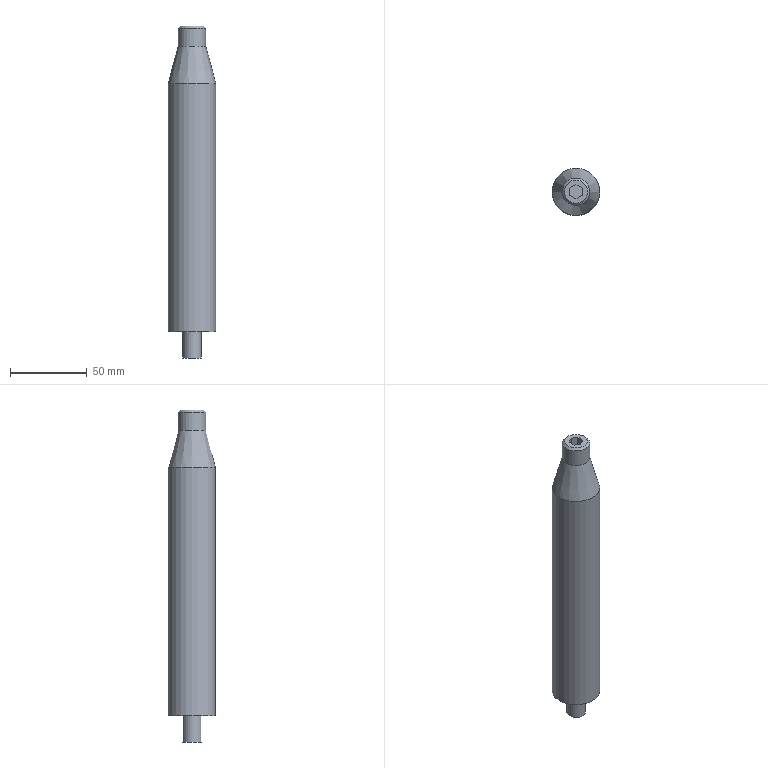Part | NX | features solid 2 | 1 solid | 15 faces | box 31 x 31 x 217 mm | volume 139271 mm3 | plane 10 | cylinder 3 | cone 2 | commonest cylinder face diameters 12 x1 18 x1 31 x1
STEP:
#1=CARTESIAN_POINT('',(-6.,-390.,130.));
#2=VERTEX_POINT('',#1);
#3=CARTESIAN_POINT('',(0.,-390.,130.));
#4=DIRECTION('',(0.,0.,-1.));
#5=DIRECTION('',(-1.,0.,0.));
#6=AXIS2_PLACEMENT_3D('',#3,#4,#5);
#7=CIRCLE('',#6,6.);
#8=EDGE_CURVE('',#2,#2,#7,.T.);
#9=ORIENTED_EDGE('',*,*,#8,.T.);
#10=EDGE_LOOP('',(#9));
#11=FACE_BOUND('',#10,.T.);
#12=CARTESIAN_POINT('',(-6.,-390.,113.));
#13=VERTEX_POINT('',#12);
#14=CARTESIAN_POINT('',(0.,-390.,113.));
#15=DIRECTION('',(0.,0.,-1.));
#16=DIRECTION('',(-1.,0.,0.));
#17=AXIS2_PLACEMENT_3D('',#14,#15,#16);
#18=CIRCLE('',#17,6.);
#19=EDGE_CURVE('',#13,#13,#18,.F.);
#20=ORIENTED_EDGE('',*,*,#19,.T.);
#21=EDGE_LOOP('',(#20));
#22=FACE_BOUND('',#21,.T.);
#23=CARTESIAN_POINT('',(0.,-390.,320.));
#24=DIRECTION('',(0.,0.,-1.));
#25=DIRECTION('',(-1.,0.,0.));
#26=AXIS2_PLACEMENT_3D('',#23,#24,#25);
#27=CYLINDRICAL_SURFACE('',#26,6.);
#28=ADVANCED_FACE('',(#11,#22),#27,.T.);
#29=ORIENTED_EDGE('',*,*,#8,.F.);
#30=EDGE_LOOP('',(#29));
#31=FACE_BOUND('',#30,.T.);
#32=CARTESIAN_POINT('',(-15.5,-390.,130.));
#33=VERTEX_POINT('',#32);
#34=CARTESIAN_POINT('',(0.,-390.,130.));
#35=DIRECTION('',(0.,0.,-1.));
#36=DIRECTION('',(-1.,0.,0.));
#37=AXIS2_PLACEMENT_3D('',#34,#35,#36);
#38=CIRCLE('',#37,15.5);
#39=EDGE_CURVE('',#33,#33,#38,.F.);
#40=ORIENTED_EDGE('',*,*,#39,.F.);
#41=EDGE_LOOP('',(#40));
#42=FACE_BOUND('',#41,.T.);
#43=CARTESIAN_POINT('',(0.,-390.,130.));
#44=DIRECTION('',(0.,0.,-1.));
#45=DIRECTION('',(-1.,0.,0.));
#46=AXIS2_PLACEMENT_3D('',#43,#44,#45);
#47=PLANE('',#46);
#48=ADVANCED_FACE('',(#31,#42),#47,.T.);
#49=CARTESIAN_POINT('',(-15.5,-390.,292.608));
#50=VERTEX_POINT('',#49);
#51=CARTESIAN_POINT('',(0.,-390.,292.608));
#52=DIRECTION('',(0.,0.,-1.));
#53=DIRECTION('',(-1.,0.,0.));
#54=AXIS2_PLACEMENT_3D('',#51,#52,#53);
#55=CIRCLE('',#54,15.5);
#56=EDGE_CURVE('',#50,#50,#55,.T.);
#57=ORIENTED_EDGE('',*,*,#56,.T.);
#58=EDGE_LOOP('',(#57));
#59=FACE_BOUND('',#58,.T.);
#60=ORIENTED_EDGE('',*,*,#39,.T.);
#61=EDGE_LOOP('',(#60));
#62=FACE_BOUND('',#61,.T.);
#63=CARTESIAN_POINT('',(0.,-390.,320.));
#64=DIRECTION('',(0.,0.,-1.));
#65=DIRECTION('',(-1.,0.,0.));
#66=AXIS2_PLACEMENT_3D('',#63,#64,#65);
#67=CYLINDRICAL_SURFACE('',#66,15.5);
#68=ADVANCED_FACE('',(#59,#62),#67,.T.);
#69=CARTESIAN_POINT('',(-9.,-390.,316.866));
#70=VERTEX_POINT('',#69);
#71=CARTESIAN_POINT('',(0.,-390.,316.866));
#72=DIRECTION('',(0.,0.,-1.));
#73=DIRECTION('',(-1.,0.,0.));
#74=AXIS2_PLACEMENT_3D('',#71,#72,#73);
#75=CIRCLE('',#74,9.);
#76=EDGE_CURVE('',#70,#70,#75,.F.);
#77=ORIENTED_EDGE('',*,*,#76,.F.);
#78=EDGE_LOOP('',(#77));
#79=FACE_BOUND('',#78,.T.);
#80=ORIENTED_EDGE('',*,*,#56,.F.);
#81=EDGE_LOOP('',(#80));
#82=FACE_BOUND('',#81,.T.);
#83=CARTESIAN_POINT('',(0.,-390.,315.));
#84=DIRECTION('',(0.,0.,-1.));
#85=DIRECTION('',(-1.,0.,0.));
#86=AXIS2_PLACEMENT_3D('',#83,#84,#85);
#87=CONICAL_SURFACE('',#86,9.5,0.2618);
#88=ADVANCED_FACE('',(#79,#82),#87,.T.);
#89=CARTESIAN_POINT('',(7.5,-390.,330.));
#90=VERTEX_POINT('',#89);
#91=CARTESIAN_POINT('',(0.,-390.,330.));
#92=DIRECTION('',(0.,0.,1.));
#93=DIRECTION('',(1.,0.,0.));
#94=AXIS2_PLACEMENT_3D('',#91,#92,#93);
#95=CIRCLE('',#94,7.5);
#96=EDGE_CURVE('',#90,#90,#95,.T.);
#97=ORIENTED_EDGE('',*,*,#96,.F.);
#98=EDGE_LOOP('',(#97));
#99=FACE_BOUND('',#98,.T.);
#100=CARTESIAN_POINT('',(-9.,-390.,328.5));
#101=VERTEX_POINT('',#100);
#102=CARTESIAN_POINT('',(0.,-390.,328.5));
#103=DIRECTION('',(0.,0.,-1.));
#104=DIRECTION('',(-1.,0.,0.));
#105=AXIS2_PLACEMENT_3D('',#102,#103,#104);
#106=CIRCLE('',#105,9.);
#107=EDGE_CURVE('',#101,#101,#106,.T.);
#108=ORIENTED_EDGE('',*,*,#107,.F.);
#109=EDGE_LOOP('',(#108));
#110=FACE_BOUND('',#109,.T.);
#111=CARTESIAN_POINT('',(0.,-390.,329.5));
#112=DIRECTION('',(0.,0.,-1.));
#113=DIRECTION('',(-1.,0.,0.));
#114=AXIS2_PLACEMENT_3D('',#111,#112,#113);
#115=CONICAL_SURFACE('',#114,8.,0.7854);
#116=ADVANCED_FACE('',(#99,#110),#115,.T.);
#117=ORIENTED_EDGE('',*,*,#107,.T.);
#118=EDGE_LOOP('',(#117));
#119=FACE_BOUND('',#118,.T.);
#120=ORIENTED_EDGE('',*,*,#76,.T.);
#121=EDGE_LOOP('',(#120));
#122=FACE_BOUND('',#121,.T.);
#123=CARTESIAN_POINT('',(0.,-390.,320.));
#124=DIRECTION('',(0.,0.,1.));
#125=DIRECTION('',(1.,0.,0.));
#126=AXIS2_PLACEMENT_3D('',#123,#124,#125);
#127=CYLINDRICAL_SURFACE('',#126,9.);
#128=ADVANCED_FACE('',(#119,#122),#127,.T.);
#129=ORIENTED_EDGE('',*,*,#96,.T.);
#130=EDGE_LOOP('',(#129));
#131=FACE_BOUND('',#130,.T.);
#132=CARTESIAN_POINT('',(0.,-394.619,330.));
#133=VERTEX_POINT('',#132);
#134=CARTESIAN_POINT('',(4.,-392.309,330.));
#135=VERTEX_POINT('',#134);
#136=CARTESIAN_POINT('',(0.2679,-394.464,330.));
#137=DIRECTION('',(-0.866,-0.5,0.));
#138=VECTOR('',#137,1000.);
#139=LINE('',#136,#138);
#140=EDGE_CURVE('',#133,#135,#139,.F.);
#141=ORIENTED_EDGE('',*,*,#140,.F.);
#142=CARTESIAN_POINT('',(-4.,-392.309,330.));
#143=VERTEX_POINT('',#142);
#144=CARTESIAN_POINT('',(-3.732,-392.464,330.));
#145=DIRECTION('',(-0.866,0.5,0.));
#146=VECTOR('',#145,1000.);
#147=LINE('',#144,#146);
#148=EDGE_CURVE('',#143,#133,#147,.F.);
#149=ORIENTED_EDGE('',*,*,#148,.F.);
#150=CARTESIAN_POINT('',(-4.,-387.691,330.));
#151=VERTEX_POINT('',#150);
#152=CARTESIAN_POINT('',(-4.,-388.,330.));
#153=DIRECTION('',(0.,-1.,0.));
#154=VECTOR('',#153,1000.);
#155=LINE('',#152,#154);
#156=EDGE_CURVE('',#151,#143,#155,.T.);
#157=ORIENTED_EDGE('',*,*,#156,.F.);
#158=CARTESIAN_POINT('',(0.,-385.381,330.));
#159=VERTEX_POINT('',#158);
#160=CARTESIAN_POINT('',(-2.,-386.536,330.));
#161=DIRECTION('',(-0.866,-0.5,0.));
#162=VECTOR('',#161,1000.);
#163=LINE('',#160,#162);
#164=EDGE_CURVE('',#151,#159,#163,.F.);
#165=ORIENTED_EDGE('',*,*,#164,.T.);
#166=CARTESIAN_POINT('',(4.,-387.691,330.));
#167=VERTEX_POINT('',#166);
#168=CARTESIAN_POINT('',(2.,-386.536,330.));
#169=DIRECTION('',(-0.866,0.5,0.));
#170=VECTOR('',#169,1000.);
#171=LINE('',#168,#170);
#172=EDGE_CURVE('',#159,#167,#171,.F.);
#173=ORIENTED_EDGE('',*,*,#172,.T.);
#174=CARTESIAN_POINT('',(4.,-388.,330.));
#175=DIRECTION('',(0.,-1.,0.));
#176=VECTOR('',#175,1000.);
#177=LINE('',#174,#176);
#178=EDGE_CURVE('',#167,#135,#177,.T.);
#179=ORIENTED_EDGE('',*,*,#178,.T.);
#180=EDGE_LOOP('',(#141,#149,#157,#165,#173,#179));
#181=FACE_BOUND('',#180,.T.);
#182=CARTESIAN_POINT('',(0.,-390.,330.));
#183=DIRECTION('',(0.,0.,1.));
#184=DIRECTION('',(1.,0.,0.));
#185=AXIS2_PLACEMENT_3D('',#182,#183,#184);
#186=PLANE('',#185);
#187=ADVANCED_FACE('',(#131,#181),#186,.T.);
#188=CARTESIAN_POINT('',(0.,-385.381,323.333));
#189=VERTEX_POINT('',#188);
#190=CARTESIAN_POINT('',(4.,-387.691,323.333));
#191=VERTEX_POINT('',#190);
#192=CARTESIAN_POINT('',(3.732,-387.536,323.333));
#193=DIRECTION('',(-0.866,0.5,0.));
#194=VECTOR('',#193,1000.);
#195=LINE('',#192,#194);
#196=EDGE_CURVE('',#189,#191,#195,.F.);
#197=ORIENTED_EDGE('',*,*,#196,.F.);
#198=CARTESIAN_POINT('',(-4.,-387.691,323.333));
#199=VERTEX_POINT('',#198);
#200=CARTESIAN_POINT('',(-0.2679,-385.536,323.333));
#201=DIRECTION('',(-0.866,-0.5,0.));
#202=VECTOR('',#201,1000.);
#203=LINE('',#200,#202);
#204=EDGE_CURVE('',#199,#189,#203,.F.);
#205=ORIENTED_EDGE('',*,*,#204,.F.);
#206=CARTESIAN_POINT('',(-4.,-392.309,323.333));
#207=VERTEX_POINT('',#206);
#208=CARTESIAN_POINT('',(-4.,-388.,323.333));
#209=DIRECTION('',(0.,-1.,0.));
#210=VECTOR('',#209,1000.);
#211=LINE('',#208,#210);
#212=EDGE_CURVE('',#199,#207,#211,.T.);
#213=ORIENTED_EDGE('',*,*,#212,.T.);
#214=CARTESIAN_POINT('',(0.,-394.619,323.333));
#215=VERTEX_POINT('',#214);
#216=CARTESIAN_POINT('',(-5.866,-391.232,323.333));
#217=DIRECTION('',(-0.866,0.5,0.));
#218=VECTOR('',#217,1000.);
#219=LINE('',#216,#218);
#220=EDGE_CURVE('',#207,#215,#219,.F.);
#221=ORIENTED_EDGE('',*,*,#220,.T.);
#222=CARTESIAN_POINT('',(4.,-392.309,323.333));
#223=VERTEX_POINT('',#222);
#224=CARTESIAN_POINT('',(-0.134,-394.696,323.333));
#225=DIRECTION('',(-0.866,-0.5,0.));
#226=VECTOR('',#225,1000.);
#227=LINE('',#224,#226);
#228=EDGE_CURVE('',#215,#223,#227,.F.);
#229=ORIENTED_EDGE('',*,*,#228,.T.);
#230=CARTESIAN_POINT('',(4.,-388.,323.333));
#231=DIRECTION('',(0.,-1.,0.));
#232=VECTOR('',#231,1000.);
#233=LINE('',#230,#232);
#234=EDGE_CURVE('',#191,#223,#233,.T.);
#235=ORIENTED_EDGE('',*,*,#234,.F.);
#236=EDGE_LOOP('',(#197,#205,#213,#221,#229,#235));
#237=FACE_BOUND('',#236,.T.);
#238=CARTESIAN_POINT('',(-4.,-388.,323.333));
#239=DIRECTION('',(0.,0.,-1.));
#240=DIRECTION('',(-1.,0.,0.));
#241=AXIS2_PLACEMENT_3D('',#238,#239,#240);
#242=PLANE('',#241);
#243=ADVANCED_FACE('',(#237),#242,.F.);
#244=ORIENTED_EDGE('',*,*,#178,.F.);
#245=CARTESIAN_POINT('',(4.,-387.691,330.));
#246=DIRECTION('',(0.,0.,1.));
#247=VECTOR('',#246,1000.);
#248=LINE('',#245,#247);
#249=EDGE_CURVE('',#167,#191,#248,.F.);
#250=ORIENTED_EDGE('',*,*,#249,.T.);
#251=ORIENTED_EDGE('',*,*,#234,.T.);
#252=CARTESIAN_POINT('',(4.,-392.309,330.));
#253=DIRECTION('',(0.,0.,1.));
#254=VECTOR('',#253,1000.);
#255=LINE('',#252,#254);
#256=EDGE_CURVE('',#135,#223,#255,.F.);
#257=ORIENTED_EDGE('',*,*,#256,.F.);
#258=EDGE_LOOP('',(#244,#250,#251,#257));
#259=FACE_BOUND('',#258,.T.);
#260=CARTESIAN_POINT('',(4.,-392.,330.));
#261=DIRECTION('',(1.,0.,0.));
#262=DIRECTION('',(0.,0.,-1.));
#263=AXIS2_PLACEMENT_3D('',#260,#261,#262);
#264=PLANE('',#263);
#265=ADVANCED_FACE('',(#259),#264,.F.);
#266=CARTESIAN_POINT('',(0.,-385.381,330.));
#267=DIRECTION('',(0.,0.,1.));
#268=VECTOR('',#267,1000.);
#269=LINE('',#266,#268);
#270=EDGE_CURVE('',#159,#189,#269,.F.);
#271=ORIENTED_EDGE('',*,*,#270,.T.);
#272=ORIENTED_EDGE('',*,*,#196,.T.);
#273=ORIENTED_EDGE('',*,*,#249,.F.);
#274=ORIENTED_EDGE('',*,*,#172,.F.);
#275=EDGE_LOOP('',(#271,#272,#273,#274));
#276=FACE_BOUND('',#275,.T.);
#277=CARTESIAN_POINT('',(3.732,-387.536,330.));
#278=DIRECTION('',(0.5,0.866,0.));
#279=DIRECTION('',(0.,0.,1.));
#280=AXIS2_PLACEMENT_3D('',#277,#278,#279);
#281=PLANE('',#280);
#282=ADVANCED_FACE('',(#276),#281,.F.);
#283=ORIENTED_EDGE('',*,*,#270,.F.);
#284=ORIENTED_EDGE('',*,*,#164,.F.);
#285=CARTESIAN_POINT('',(-4.,-387.691,330.));
#286=DIRECTION('',(0.,0.,1.));
#287=VECTOR('',#286,1000.);
#288=LINE('',#285,#287);
#289=EDGE_CURVE('',#151,#199,#288,.F.);
#290=ORIENTED_EDGE('',*,*,#289,.T.);
#291=ORIENTED_EDGE('',*,*,#204,.T.);
#292=EDGE_LOOP('',(#283,#284,#290,#291));
#293=FACE_BOUND('',#292,.T.);
#294=CARTESIAN_POINT('',(-0.2679,-385.536,330.));
#295=DIRECTION('',(-0.5,0.866,0.));
#296=DIRECTION('',(0.,0.,-1.));
#297=AXIS2_PLACEMENT_3D('',#294,#295,#296);
#298=PLANE('',#297);
#299=ADVANCED_FACE('',(#293),#298,.F.);
#300=ORIENTED_EDGE('',*,*,#156,.T.);
#301=CARTESIAN_POINT('',(-4.,-392.309,330.));
#302=DIRECTION('',(0.,0.,1.));
#303=VECTOR('',#302,1000.);
#304=LINE('',#301,#303);
#305=EDGE_CURVE('',#143,#207,#304,.F.);
#306=ORIENTED_EDGE('',*,*,#305,.T.);
#307=ORIENTED_EDGE('',*,*,#212,.F.);
#308=ORIENTED_EDGE('',*,*,#289,.F.);
#309=EDGE_LOOP('',(#300,#306,#307,#308));
#310=FACE_BOUND('',#309,.T.);
#311=CARTESIAN_POINT('',(-4.,-388.,330.));
#312=DIRECTION('',(-1.,0.,0.));
#313=DIRECTION('',(0.,0.,1.));
#314=AXIS2_PLACEMENT_3D('',#311,#312,#313);
#315=PLANE('',#314);
#316=ADVANCED_FACE('',(#310),#315,.F.);
#317=CARTESIAN_POINT('',(0.,-394.619,330.));
#318=DIRECTION('',(0.,0.,1.));
#319=VECTOR('',#318,1000.);
#320=LINE('',#317,#319);
#321=EDGE_CURVE('',#133,#215,#320,.F.);
#322=ORIENTED_EDGE('',*,*,#321,.T.);
#323=ORIENTED_EDGE('',*,*,#220,.F.);
#324=ORIENTED_EDGE('',*,*,#305,.F.);
#325=ORIENTED_EDGE('',*,*,#148,.T.);
#326=EDGE_LOOP('',(#322,#323,#324,#325));
#327=FACE_BOUND('',#326,.T.);
#328=CARTESIAN_POINT('',(-3.732,-392.464,330.));
#329=DIRECTION('',(-0.5,-0.866,0.));
#330=DIRECTION('',(0.,0.,-1.));
#331=AXIS2_PLACEMENT_3D('',#328,#329,#330);
#332=PLANE('',#331);
#333=ADVANCED_FACE('',(#327),#332,.F.);
#334=ORIENTED_EDGE('',*,*,#321,.F.);
#335=ORIENTED_EDGE('',*,*,#140,.T.);
#336=ORIENTED_EDGE('',*,*,#256,.T.);
#337=ORIENTED_EDGE('',*,*,#228,.F.);
#338=EDGE_LOOP('',(#334,#335,#336,#337));
#339=FACE_BOUND('',#338,.T.);
#340=CARTESIAN_POINT('',(0.2679,-394.464,330.));
#341=DIRECTION('',(0.5,-0.866,0.));
#342=DIRECTION('',(0.,0.,1.));
#343=AXIS2_PLACEMENT_3D('',#340,#341,#342);
#344=PLANE('',#343);
#345=ADVANCED_FACE('',(#339),#344,.F.);
#346=ORIENTED_EDGE('',*,*,#19,.F.);
#347=EDGE_LOOP('',(#346));
#348=FACE_BOUND('',#347,.T.);
#349=CARTESIAN_POINT('',(0.,-390.,113.));
#350=DIRECTION('',(0.,0.,-1.));
#351=DIRECTION('',(-1.,0.,0.));
#352=AXIS2_PLACEMENT_3D('',#349,#350,#351);
#353=PLANE('',#352);
#354=ADVANCED_FACE('',(#348),#353,.T.);
#355=CLOSED_SHELL('',(#28,#48,#68,#88,#116,#128,#187,#243,#265,#282,#299,#316,#333,#345,#354));
#356=MANIFOLD_SOLID_BREP('',#355);
#357=(LENGTH_UNIT()NAMED_UNIT(*)SI_UNIT(.MILLI.,.METRE.));
#358=UNCERTAINTY_MEASURE_WITH_UNIT(LENGTH_MEASURE(0.00001),#357,'','');
#359=(NAMED_UNIT(*)PLANE_ANGLE_UNIT()SI_UNIT($,.RADIAN.));
#360=(NAMED_UNIT(*)SI_UNIT($,.STERADIAN.)SOLID_ANGLE_UNIT());
#361=(GEOMETRIC_REPRESENTATION_CONTEXT(3)GLOBAL_UNCERTAINTY_ASSIGNED_CONTEXT((#358))GLOBAL_UNIT_ASSIGNED_CONTEXT((#357,#359,#360))REPRESENTATION_CONTEXT('',''));
#362=ADVANCED_BREP_SHAPE_REPRESENTATION('',(#356),#361);